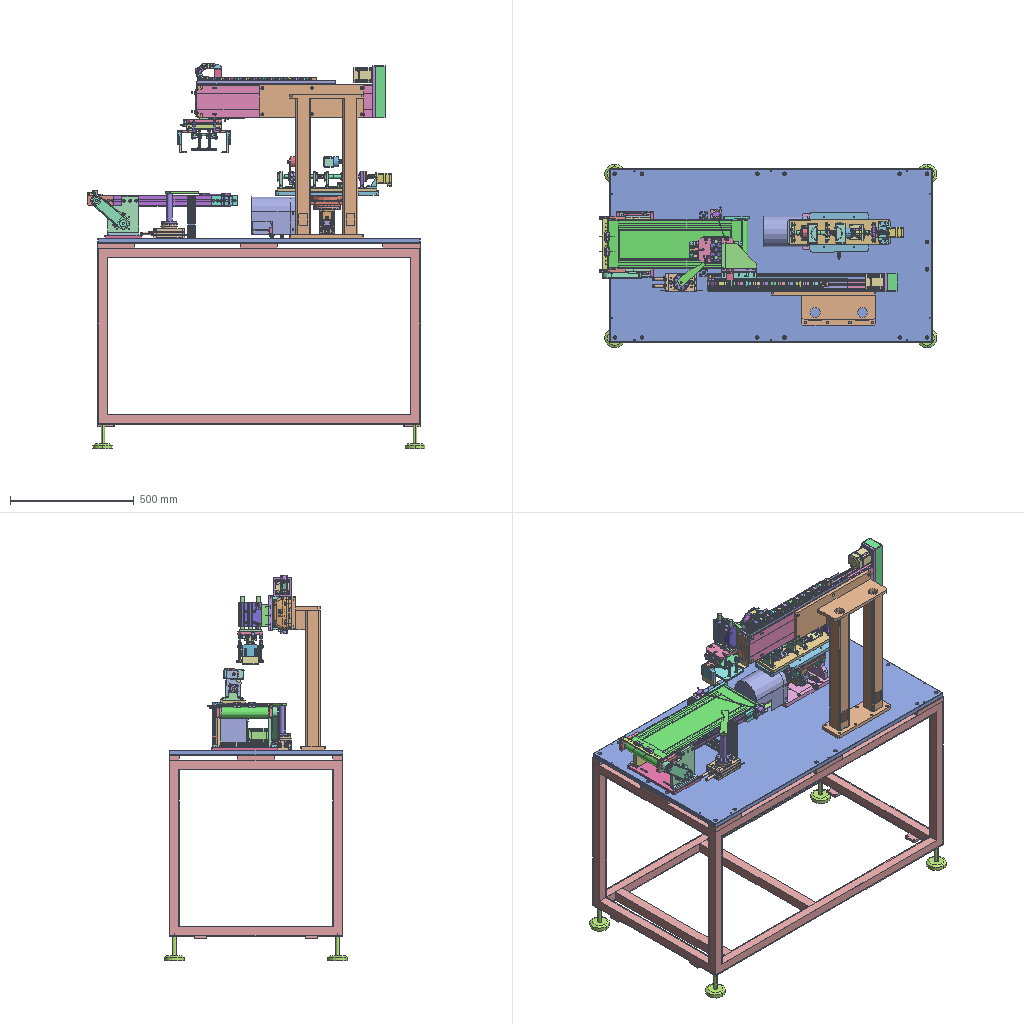Assembly | SolidWorks | 144 different items | 252 placed | box 1362 x 740 x 1556 mm
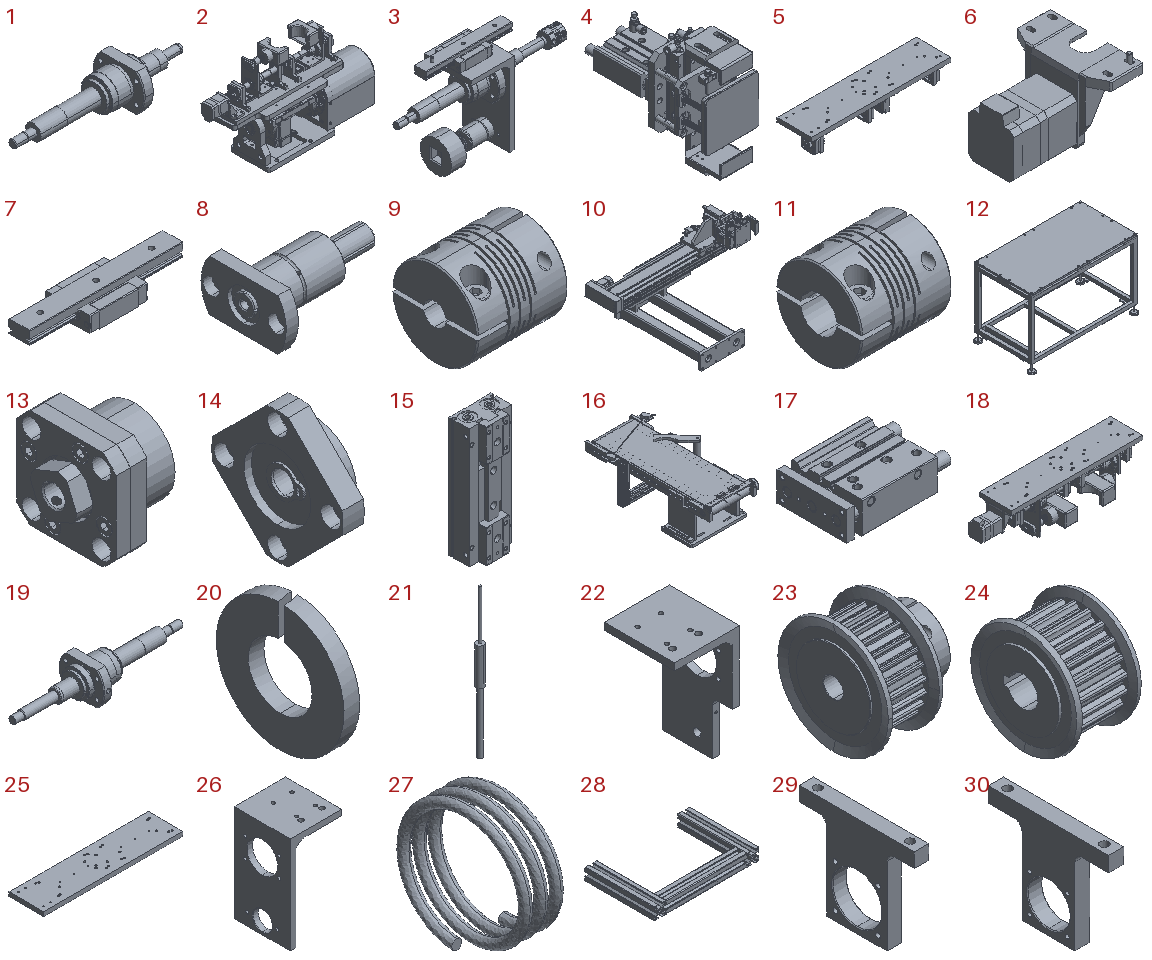Parts list (item | name | quantity | parent item | size | volume | features):
1 | (subassembly) | x1 | in 18 | 171 x 53 x 38 mm | 62164 mm3 | features AEMSimFeature 1
2 | (subassembly) | x1 | - | - | 4755058 mm3 | features CompositeCurve 2, ReferencePattern 2, MirrorCompFeat 1
3 | (subassembly) | x1 | in 18 | 209.2 x 60 x 132 mm | 185380 mm3 | features AEMSimFeature 1, CompositeCurve 1
4 | (subassembly) | x1 | in 10 | 110 x 275 x 215 mm | 1117896 mm3 | features CompositeCurve 3
5 | (subassembly) | x1 | in 18 | 400 x 100 x 81 mm | 622322 mm3 | features AEMSimFeature 1
6 | (subassembly) | x1 | in 18 | 99 x 88 x 69 mm | 136983 mm3 | features AEMSimFeature 1
7 | (subassembly) | x2 | in 3, 18 | 110 x 32 x 16 mm | 26387 mm3 | features AEMSimFeature 1
8 | (subassembly) | x1 | in 3 | 60 x 42 x 25 mm | 18059 mm3 | features AEMSimFeature 1
9 | (subassembly) | x1 | in 3 | 20 x 19 x 19 mm | 4000 mm3 | features AEMSimFeature 1
10 | (subassembly) | x1 | - | - | 8279258 mm3 | -
11 | (subassembly) | x1 | in 18 | 20 x 19 x 19 mm | 3812 mm3 | features AEMSimFeature 1
12 | (subassembly) | x1 | - | 1340 x 740 x 850 mm | 26625287 mm3 | -
13 | (subassembly) | x1 | in 5 | 34.5 x 42 x 42 mm | 32034 mm3 | features AEMSimFeature 1
14 | (subassembly) | x3 | in 5 | 12 x 43 x 43 mm | 8481 mm3 | features AEMSimFeature 1
15 | (subassembly) | x1 | in 4 | 50 x 33 x 142.8 mm | 178016 mm3 | -
16 | (subassembly) | x1 | - | 341.242 x 608 x 194 mm | 3807231 mm3 | features Belt 1
17 | (subassembly) | x1 | in 4 | 142 x 93 x 42 mm | 365239 mm3 | -
18 | (subassembly) | x1 | in 2 | - | 1293275 mm3 | features AEMSimFeature 1, CompositeCurve 1, MateUpdatePoint 1
19 | (subassembly) | x1 | in 3 | 196 x 53 x 38 mm | 63498 mm3 | features AEMSimFeature 1
20 | - | x1 | in 18 | 1.5 x 12.2 x 12.197 mm | 128.674 mm3 | features BaseBody 1
21 | - | x2 | in 16 | 3 x 3 x 60 mm | 185.354 mm3 | features BaseBody 1
22 | - | x1 | in 18 | 55 x 60 x 104 mm | 45466 mm3 | features ICE 5, HoleWzd 3, Fillet 2, Extrusion 1
23 | - | x1 | in 16 | - | - | features BaseBody 1, RefSurface 1
24 | - | x1 | in 16 | 22 x 36 x 36 mm | 13176 mm3 | features BaseBody 1
25 | - | x1 | in 5 | 400 x 100 x 12 mm | 474136 mm3 | features HoleWzd 4, Extrusion 1, ICE 1
26 | - | x1 | in 3 | 55 x 60 x 104 mm | 48156 mm3 | features ICE 3, HoleWzd 2, Chamfer 1, Extrusion 1, Fillet 1
27 | - | x2 | in 3 | 7.3 x 16 x 16 mm | 183.83 mm3 | features BaseBody 1, RefAxis 1
28 | - | x1 | in 16 | 260 x 171 x 30 mm | 182154 mm3 | features WeldMemberFeat 1, WeldmentFeature 1
29 | - | x1 | in 5 | 10 x 80 x 69 mm | 22964 mm3 | features HoleWzd 2, Chamfer 1, Extrusion 1, Fillet 1, ICE 1
30 | - | x3 | in 5 | 10 x 80 x 66 mm | 20856 mm3 | features HoleWzd 2, Chamfer 1, Extrusion 1, Fillet 1, ICE 1
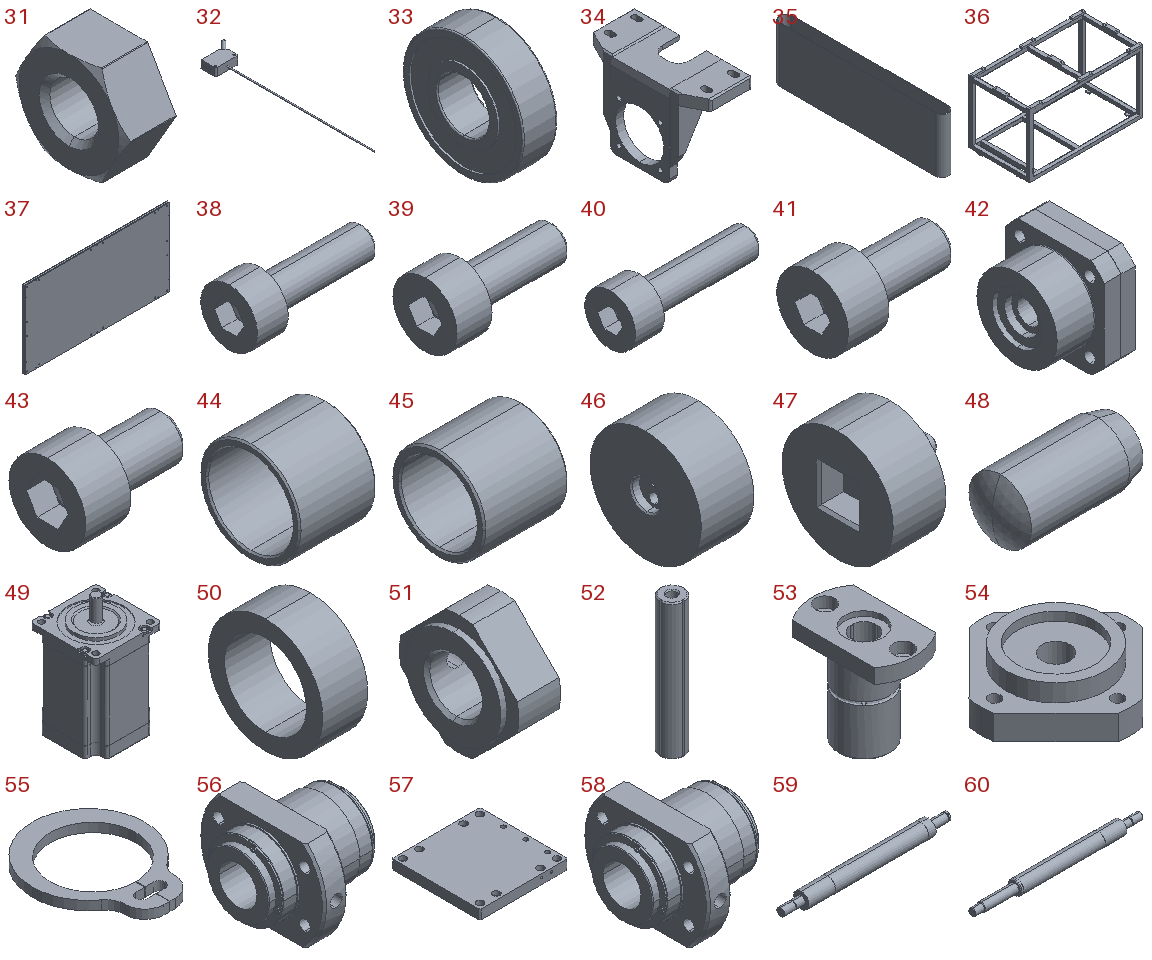31 | - | x1 | in 18 | 5 x 11.5 x 10 mm | 332.083 mm3 | features BaseBody 1
32 | - | x2 | in 16 | 44.556 x 232.556 x 10.8 mm | 6994 mm3 | features BaseBody 1
33 | - | x4 | in 16 | 8 x 28 x 28 mm | 3776 mm3 | features BaseBody 1
34 | - | x1 | in 6 | 40 x 88 x 62 mm | 31074 mm3 | features ICE 9, Chamfer 4, Fillet 3, Extrusion 1, HoleWzd 1
35 | - | x1 | in 16 | 44.5 x 584.5 x 190 mm | 461137 mm3 | features BeltProfileFeature 1, ExtruThin 1
36 | - | x1 | in 12 | 1300 x 700 x 740 mm | 7989139 mm3 | features ICE 11, MirrorPattern 9, HoleWzd 5, LPattern 5, 3DProfileFeature 4, Chamfer 1, Extrusion 1, Shell 1
37 | - | x1 | in 12 | 1300 x 20 x 700 mm | 18144468 mm3 | features MirrorPattern 5, 3DProfileFeature 4, HoleWzd 4, LPattern 4, Chamfer 1, Extrusion 1
38 | - | x8 | in 3, 5, 6, 18 | 13 x 5.5 x 5.5 mm | 132.881 mm3 | features BaseBody 1
39 | - | x1 | in 3 | 11 x 5.5 x 5.5 mm | 118.744 mm3 | features BaseBody 1
40 | - | x4 | in 3, 5, 6, 18 | 19 x 7 x 7 mm | 324.822 mm3 | features BaseBody 1
41 | - | x1 | in 3 | 12 x 7 x 7 mm | 236.857 mm3 | features BaseBody 1
42 | - | x1 | in 13 | 29 x 42 x 42 mm | 30074 mm3 | features BaseBody 1
43 | - | x1 | in 3 | 13 x 8.5 x 8.5 mm | 402.153 mm3 | features BaseBody 1
44 | - | x1 | in 3 | 10 x 13 x 13 mm | 373.975 mm3 | features BaseBody 1
45 | - | x1 | in 18 | 10 x 11 x 11 mm | 311.646 mm3 | features BaseBody 1
46 | - | x1 | in 3 | 19 x 40 x 40 mm | 21751 mm3 | features ICE 3, Chamfer 2, HoleWzd 1, Revolution 1
47 | - | x1 | in 18 | 33 x 40 x 40 mm | 22559 mm3 | features Chamfer 2, ICE 2, Revolution 1
48 | - | x16 | in 3, 5, 18 | 10 x 5 x 5 mm | 185.449 mm3 | features Revolution 1
49 | - | x1 | in 16 | 57.15 x 58.15 x 100.6 mm | 235224 mm3 | features BaseBody 2
50 | - | x1 | in 13 | 5.5 x 14 x 14 mm | 414.69 mm3 | features BaseBody 1
51 | - | x1 | in 13 | 8 x 20 x 20 mm | 1546 mm3 | features BaseBody 1
52 | - | x1 | in 8 | 10.348 x 10.348 x 60 mm | 4741 mm3 | features BaseBody 1
53 | - | x1 | in 8 | 25 x 42 x 40 mm | 13318 mm3 | features BaseBody 1
54 | - | x3 | in 14 | 43 x 43 x 12 mm | 8449 mm3 | features BaseBody 1
55 | - | x3 | in 14 | 10 x 12.2 x 0.8 mm | 32.103 mm3 | features BaseBody 1
56 | - | x1 | in 19 | 45 x 53 x 38 mm | 34023 mm3 | features ICE 5, CirPattern 2, HoleWzd 2, Chamfer 1, Fillet 1, RevCut 1, Revolution 1
57 | - | x1 | in 10 | 140 x 140 x 15 mm | 283192 mm3 | features HoleWzd 3, Chamfer 1, Extrusion 1, LPattern 1, MirrorPattern 1
58 | - | x1 | in 1 | 45 x 53 x 38 mm | 34023 mm3 | features ICE 5, CirPattern 2, HoleWzd 2, Chamfer 1, Fillet 1, RevCut 1, Revolution 1
59 | - | x1 | in 1 | 171 x 16 x 16 mm | 28140 mm3 | features Chamfer 1, RevCut 1, Revolution 1
60 | - | x1 | in 19 | 196 x 16 x 16 mm | 29474 mm3 | features Chamfer 2, RevCut 1, Revolution 1
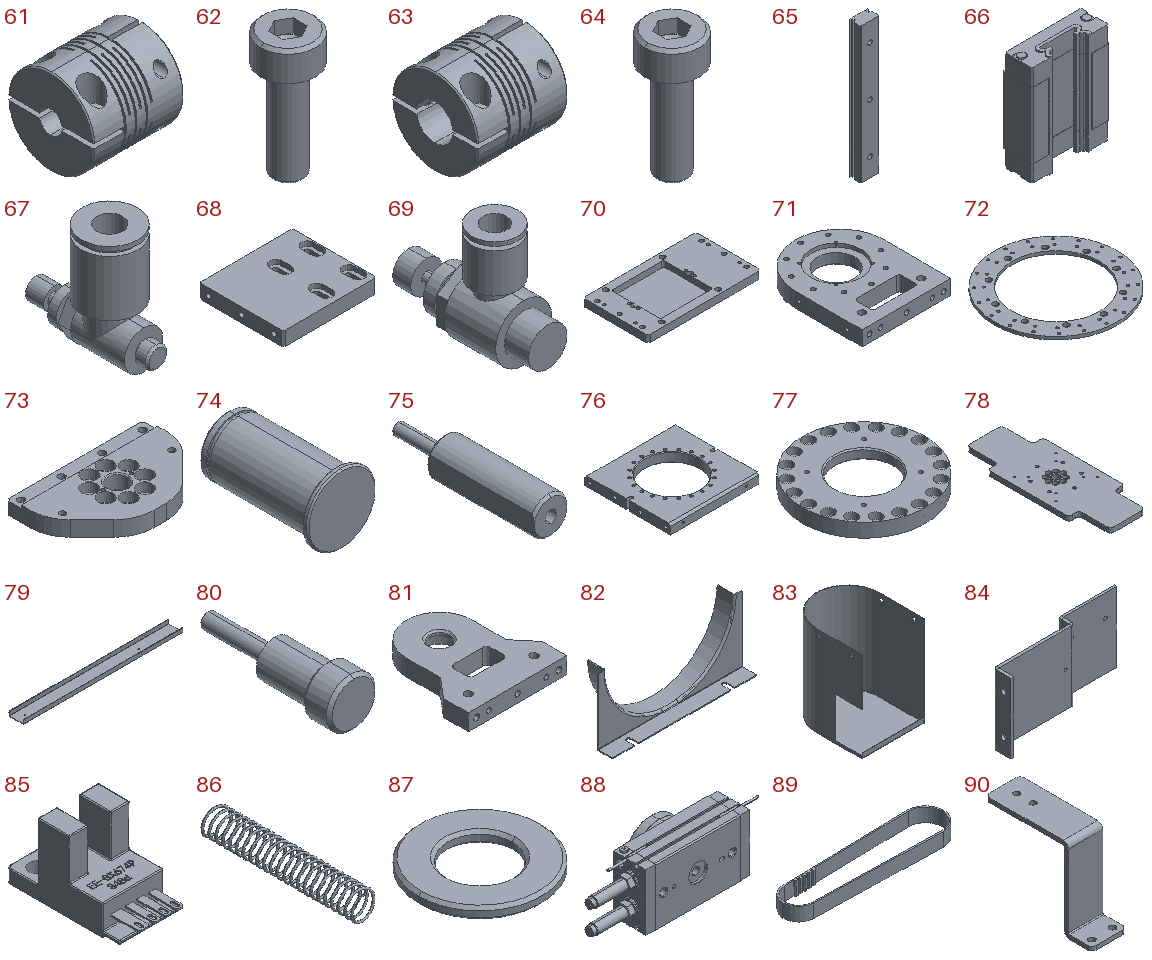61 | - | x1 | in 9 | 20 x 19 x 19 mm | 3713 mm3 | features BaseBody 1
62 | - | x4 | in 9 | 4.5 x 4.5 x 10.36 mm | 71.746 mm3 | features BaseBody 1
63 | - | x1 | in 11 | 20 x 19 x 19 mm | 3525 mm3 | features BaseBody 1
64 | - | x4 | in 11 | 4.5 x 4.5 x 10.36 mm | 71.746 mm3 | features BaseBody 1
65 | - | x2 | in 7 | 15 x 9.5 x 110 mm | 14060 mm3 | features BaseBody 1
66 | - | x2 | in 7 | 32 x 12 x 42.4 mm | 12327 mm3 | features BaseBody 1
67 | - | x2 | in 4 | 13 x 28.3 x 26 mm | 2880 mm3 | features BaseBody 1
68 | - | x1 | in 10 | 100 x 90 x 15 mm | 125181 mm3 | features ICE 2, Chamfer 1, Extrusion 1, HoleWzd 1, LPattern 1
69 | - | x2 | in 4 | 14.2 x 35.2 x 27.5 mm | 4410 mm3 | features BaseBody 1
70 | - | x1 | in 2 | 252 x 145 x 16 mm | 394345 mm3 | features HoleWzd 5, Chamfer 1, Extrusion 1, ICE 1, MirrorPattern 1
71 | - | x1 | in 2 | 120 x 150 x 20 mm | 234004 mm3 | features HoleWzd 6, CirPattern 2, ICE 2, Chamfer 1, Extrusion 1, MirrorPattern 1
72 | - | x2 | in 2 | 123 x 123 x 3 mm | 16511 mm3 | features CirPattern 2, HoleWzd 2, Extrusion 1
73 | - | x2 | in 2 | 135 x 85 x 15 mm | 108283 mm3 | features HoleWzd 5, Chamfer 2, CirPattern 1, Extrusion 1, ICE 1
74 | - | x2 | in 2 | 24 x 40 x 24 mm | 12725 mm3 | features Revolution 1
75 | - | x2 | in 2 | 7 x 33 x 8 mm | 1085 mm3 | features Chamfer 2, Fillet 1, HoleWzd 1, ICE 1, Revolution 1
76 | - | x1 | in 2 | 140 x 135 x 15 mm | 184976 mm3 | features HoleWzd 3, Chamfer 2, MirrorPattern 2, CirPattern 1, Extrusion 1, ICE 1
77 | - | x1 | in 2 | 107 x 107 x 12 mm | 66155 mm3 | features CirPattern 2, HoleWzd 2, Chamfer 1, Extrusion 1, ICE 1
78 | - | x1 | in 2 | 160 x 415 x 14 mm | 752880 mm3 | features HoleWzd 3, CirPattern 2, ICE 2, Chamfer 1, Extrusion 1, Fillet 1, MirrorPattern 1
79 | - | x1 | in 10 | 560 x 52 x 15 mm | 65239 mm3 | features ICE 2, EdgeFlange 1, Fillet 1, FlatPattern 1, HoleWzd 1, LPattern 1, SMBaseFlange 1, SheetMetal 1
80 | - | x1 | in 2 | 8 x 24 x 8 mm | 516.339 mm3 | features Chamfer 2, Fillet 1, Revolution 1
81 | - | x1 | in 2 | 120 x 135 x 20 mm | 181137 mm3 | features HoleWzd 3, ICE 2, Chamfer 1, Extrusion 1
82 | - | x2 | in 2 | 150 x 33 x 69 mm | 8933 mm3 | features ICE 3, Fillet 2, EdgeFlange 1, FlatPattern 1, SMBaseFlange 1, SheetMetal 1
83 | - | x1 | in 2 | 124 x 152 x 178 mm | 79554 mm3 | features EdgeFlange 3, ICE 2, 3DProfileFeature 1, FlatPattern 1, SMBaseFlange 1, SheetMetal 1
84 | - | x1 | in 2 | 151 x 33 x 80 mm | 42488 mm3 | features EdgeFlange 3, HoleWzd 3, FlatPattern 1, SMBaseFlange 1, SheetMetal 1
85 | - | x6 | in 2 | 13.6 x 28 x 16 mm | 2162 mm3 | features ICE 6, Fillet 3, Chamfer 1, Extrusion 1, HoleWzd 1
86 | - | x4 | in 4 | 8 x 45 x 8 mm | 146.9 mm3 | features Helix 1, ICE 1, Sweep 1
87 | - | x1 | in 3 | 21 x 21 x 2 mm | 477.522 mm3 | features BaseBody 1
88 | - | x1 | in 16 | 200 x 57 x 74 mm | 397497 mm3 | features BaseBody 3
89 | - | x1 | in 16 | 177.014 x 40.237 x 15 mm | 9222 mm3 | features BaseBody 1
90 | - | x1 | in 10 | 25 x 77 x 60 mm | 9704 mm3 | features EdgeFlange 2, HoleWzd 2, Fillet 1, FlatPattern 1, SMBaseFlange 1, SheetMetal 1
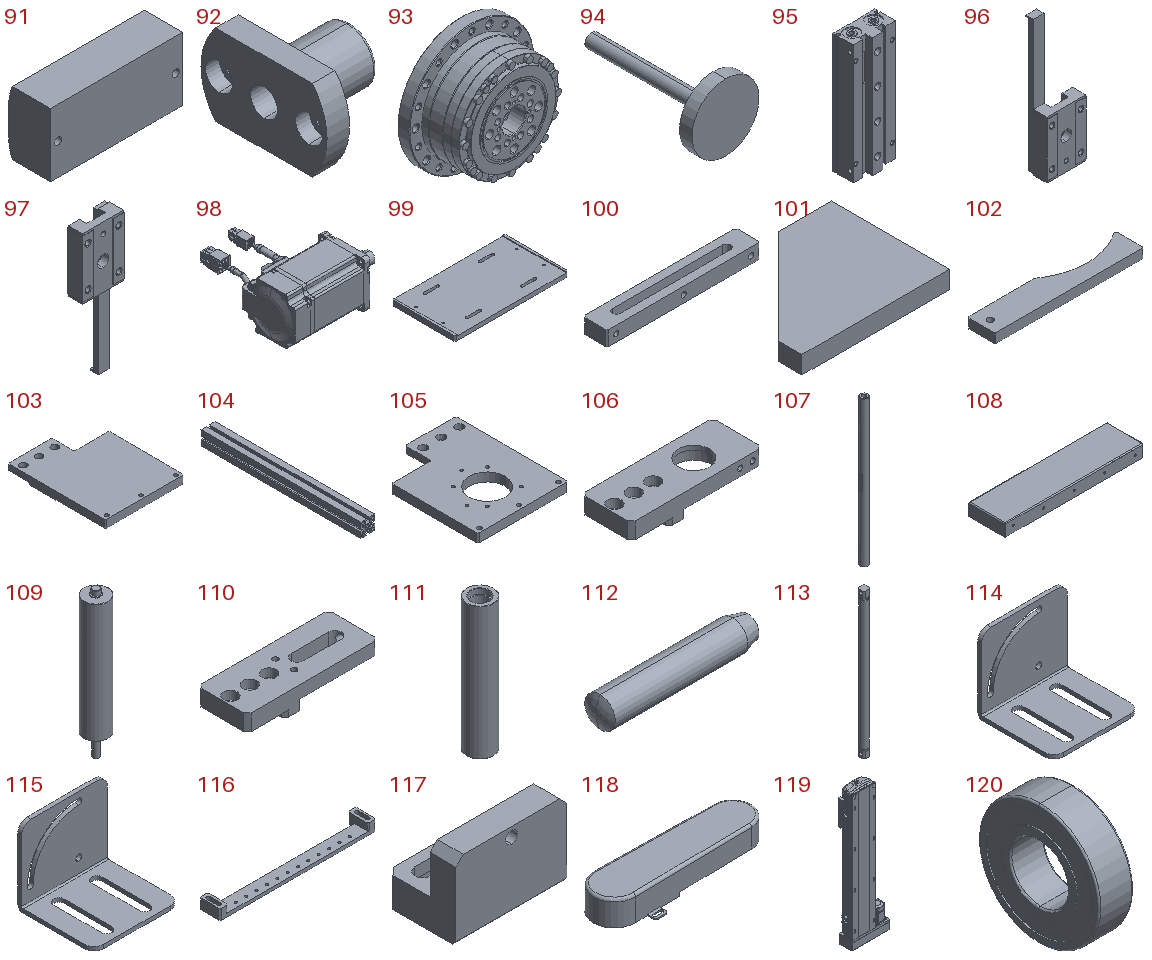91 | - | x1 | in 2 | 77.96 x 24.63 x 37.4 mm | 70032 mm3 | features ICE 3, Extrusion 1
92 | - | x4 | in 4 | 19 x 28 x 18 mm | 3154 mm3 | features RevCut 2, ICE 1, Revolution 1
93 | - | x2 | in 2 | 107 x 52 x 107 mm | 219965 mm3 | features BaseBody 45
94 | - | x4 | in 12 | 80 x 160 x 80 mm | 122920 mm3 | features Revolution 1
95 | - | x1 | in 15 | 50 x 28.3 x 142 mm | 158930 mm3 | features BaseBody 1
96 | - | x1 | in 15 | 27 x 14.6 x 93.2 mm | 9543 mm3 | features BaseBody 1
97 | - | x1 | in 15 | 27 x 14.6 x 93.2 mm | 9543 mm3 | features BaseBody 1
98 | - | x2 | in 2 | 129 x 145.682 x 60 mm | 347582 mm3 | features BaseBody 7
99 | - | x1 | in 16 | 268 x 150 x 12 mm | 394710 mm3 | features ICE 2, Chamfer 1, Extrusion 1, HoleWzd 1
100 | - | x2 | in 16 | 125 x 20 x 12 mm | 22020 mm3 | features Chamfer 2, Extrusion 1, HoleWzd 1, ICE 1
101 | - | x1 | in 10 | 125 x 100 x 15 mm | 139500 mm3 | features Chamfer 1, Extrusion 1
102 | - | x1 | in 16 | 160 x 30 x 10 mm | 39472 mm3 | features Chamfer 2, Extrusion 1, HoleWzd 1, ICE 1
103 | - | x1 | in 16 | 125 x 156 x 12 mm | 198828 mm3 | features HoleWzd 2, ICE 2, Chamfer 1, Extrusion 1, Fillet 1
104 | - | x2 | in 16 | 40 x 455 x 40 mm | 322038 mm3 | features WeldMemberFeat 1, WeldmentFeature 1
105 | - | x1 | in 16 | 125 x 156 x 12 mm | 174396 mm3 | features HoleWzd 4, ICE 3, Chamfer 1, Extrusion 1, Fillet 1
106 | - | x2 | in 16 | 105 x 40 x 18 mm | 43487 mm3 | features ICE 5, HoleWzd 2, Chamfer 1, Extrusion 1, MirrorPattern 1
107 | - | x2 | in 16 | 10 x 10 x 194 mm | 14513 mm3 | features HoleWzd 2, Chamfer 1, Extrusion 1, ICE 1
108 | - | x1 | in 16 | 455 x 120 x 40 mm | 145562 mm3 | features Extrusion 1, Fillet 1, HoleWzd 1, Shell 1
109 | - | x1 | in 16 | 40.5 x 40.5 x 246 mm | 261959 mm3 | features ICE 6, Chamfer 1, Extrusion 1, Fillet 1
110 | - | x2 | in 16 | 105 x 40 x 18 mm | 42827 mm3 | features HoleWzd 3, ICE 3, Chamfer 1, Cut 1, Extrusion 1
111 | - | x1 | in 16 | 40.5 x 40.5 x 200 mm | 157423 mm3 | features ICE 2, Chamfer 1, Extrusion 1, MirrorPattern 1
112 | - | x2 | in 3, 18 | 10 x 2 x 2 mm | 30.238 mm3 | features Revolution 1
113 | - | x1 | in 16 | 12 x 12 x 226 mm | 24710 mm3 | features Extrusion 1, HoleWzd 1, ICE 1, MirrorPattern 1, RevCut 1
114 | - | x1 | in 16 | 45 x 40 x 40 mm | 5977 mm3 | features ICE 2, EdgeFlange 1, Fillet 1, FlatPattern 1, HoleWzd 1, SMBaseFlange 1, SheetMetal 1
115 | - | x1 | in 16 | 45 x 40 x 40 mm | 5977 mm3 | features ICE 2, EdgeFlange 1, Fillet 1, FlatPattern 1, HoleWzd 1, SMBaseFlange 1, SheetMetal 1
116 | - | x1 | in 16 | 226 x 30 x 15 mm | 25281 mm3 | features ICE 4, Chamfer 1, Extrusion 1, Fillet 1, HoleWzd 1, LPattern 1
117 | - | x2 | in 16 | 30 x 19 x 20.5 mm | 5581 mm3 | features ICE 4, Chamfer 2, HoleWzd 2, Extrusion 1
118 | - | x1 | in 16 | 189.5 x 70 x 30 mm | 29758 mm3 | features ICE 3, Extrusion 1, Fillet 1, MirrorPattern 1, Shell 1
119 | - | x1 | in 10 | 224 x 78.028 x 768.474 mm | 3697252 mm3 | features BaseBody 11
120 | - | x1 | in 2 | 12 x 42 x 42 mm | 12378 mm3 | features RefAxis 9, 3DProfileFeature 3, Revolution 1
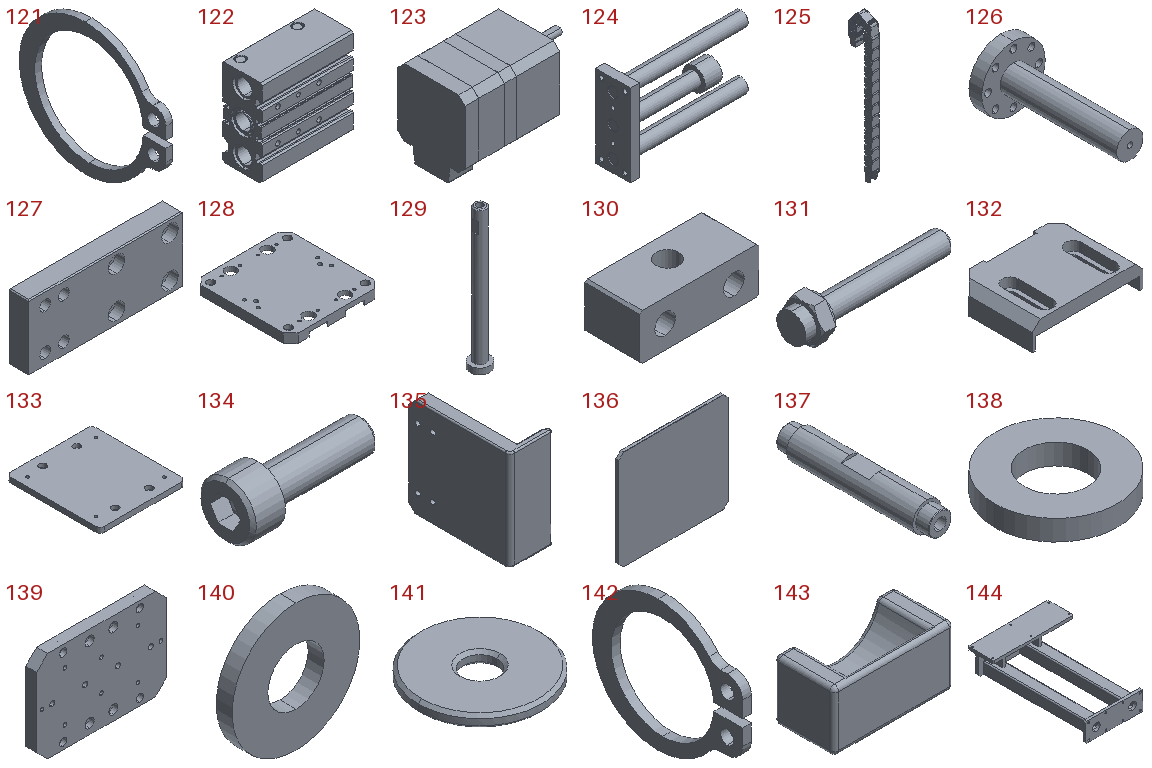121 | - | x1 | in 2 | 1.2 x 25.6 x 23.05 mm | 179.471 mm3 | features RefAxis 6, 3DProfileFeature 2, Extrusion 1, ICE 1
122 | - | x1 | in 17 | 97.5 x 42 x 93 mm | 253511 mm3 | features BaseBody 1
123 | - | x1 | in 6 | 79 x 42 x 51 mm | 105451 mm3 | features ICE 8, Chamfer 1, Extrusion 1, Fillet 1, HoleWzd 1, Revolution 1
124 | - | x1 | in 17 | 142 x 38 x 91 mm | 111727 mm3 | features BaseBody 1
125 | - | x1 | in 10 | 29.1 x 79.262 x 491.255 mm | 146687 mm3 | features BaseBody 18
126 | - | x1 | in 16 | 60 x 126 x 60 mm | 87403 mm3 | features HoleWzd 3, Cut 1, Extrusion 1, ICE 1
127 | - | x2 | in 4 | 75 x 10 x 32 mm | 18437 mm3 | features ICE 3, HoleWzd 2, Chamfer 1, Extrusion 1
128 | - | x1 | in 4 | 100 x 106 x 10 mm | 85872 mm3 | features HoleWzd 4, ICE 3, Chamfer 1, Extrusion 1, MirrorPattern 1
129 | - | x4 | in 4 | 10 x 10 x 71 mm | 2041 mm3 | features ICE 2, Chamfer 1, Extrusion 1, HoleWzd 1
130 | - | x2 | in 4 | 26 x 12 x 10 mm | 2220 mm3 | features HoleWzd 2, Chamfer 1, Extrusion 1
131 | - | x2 | in 4 | 42.15 x 11.547 x 10 mm | 1487 mm3 | features RevCut 4, ICE 2, Chamfer 1, Extrusion 1, Fillet 1, LPattern 1, Revolution 1
132 | - | x2 | in 4 | 70 x 50 x 16 mm | 29528 mm3 | features ICE 4, Chamfer 2, Extrusion 1, HoleWzd 1
133 | - | x1 | in 4 | 100 x 110 x 6 mm | 64666 mm3 | features HoleWzd 2, Extrusion 1, Fillet 1
134 | - | x4 | in 5 | 21 x 8.5 x 8.5 mm | 556.026 mm3 | features BaseBody 1
135 | - | x2 | in 4 | 28 x 67 x 66 mm | 39840 mm3 | features Fillet 3, Chamfer 2, Extrusion 1, HoleWzd 1
136 | - | x1 | in 4 | 110 x 3 x 100 mm | 32835 mm3 | features Chamfer 2, Extrusion 1, HoleWzd 1
137 | - | x4 | in 4 | 10 x 53 x 10 mm | 3526 mm3 | features ICE 3, Chamfer 1, HoleWzd 1, MirrorPattern 1, Revolution 1
138 | - | x8 | in 4 | 12 x 12 x 2 mm | 165.813 mm3 | features Extrusion 1
139 | - | x1 | in 4 | 142 x 12 x 100 mm | 155775 mm3 | features HoleWzd 6, Chamfer 1, Extrusion 1, ICE 1
140 | - | x8 | in 4 | 12 x 1.5 x 12 mm | 136.553 mm3 | features FlatPattern 1, SMBaseFlange 1, SheetMetal 1
141 | - | x1 | in 3 | 20 x 20 x 2 mm | 560.774 mm3 | features BaseBody 1
142 | - | x2 | in 16 | 1 x 16.8 x 14.65 mm | 77.172 mm3 | features BaseBody 1
143 | - | x2 | in 18 | 80 x 40 x 40 mm | 93219 mm3 | features Extrusion 1, Fillet 1, ICE 1
144 | - | x1 | in 10 | 420 x 620 x 135 mm | 2694672 mm3 | features ICE 7, Chamfer 3, LPattern 2, Extrusion 1, HoleWzd 1
Mates (type | each side: item.copy, entity, surface, feature), first 302 of 527 lines:
In the top assembly
Coincident | 37.1 face plane Boss-Extrude 1 | 70.1 face plane Boss-Extrude 1
Coincident | 37.1 face plane Boss-Extrude 1 | 144.1 face plane Boss-Extrude 1
DistanceDim | 144.1 face plane Boss-Extrude 1 | 37.1 face plane Boss-Extrude 1 | 2 times
DistanceDim | 70.1 face plane Boss-Extrude 1 | 36.1 face plane Boss-Extrude 1
DistanceDim | 81.1 face plane Boss-Extrude 1 | 37.1 face plane Boss-Extrude 1
Coincident | 37.1 face plane Boss-Extrude 1 | 99.1 face plane Boss-Extrude 1
DistanceDim | 99.1 face plane Boss-Extrude 1 | 36.1 face plane Boss-Extrude 1
DistanceDim | 103.1 face plane Boss-Extrude 1 | 37.1 face plane Boss-Extrude 1
In subassembly 12
DistanceDim | 36.2 face plane Boss-Extrude 1 | 37.2 face plane Boss-Extrude 1
Coincident | 36.2 face plane Boss-Extrude 1 | 37.2 face plane Boss-Extrude 1 | 2 times
DistanceDim | 94.1 face plane Revolve 1 | 36.2 face plane Boss-Extrude 2
Concentric | 36.2 face cylinder Mirror 3 | 94.1 face cylinder Revolve 1
Coincident | 94.1 face plane Revolve 1 | 94.2 face plane Revolve 1
Coincident | 94.1 face plane Revolve 1 | 94.3 face plane Revolve 1
Coincident | 94.2 face plane Revolve 1 | 94.4 face plane Revolve 1
Concentric | 36.2 face cylinder Mirror 4 | 94.4 face cylinder Revolve 1
Concentric | 36.2 face cylinder Mirror 4 | 94.2 face cylinder Revolve 1
Concentric | 36.2 face cylinder Boss-Extrude 8 | 94.3 face cylinder Revolve 1
In subassembly 16
Coincident | 100.1 face plane Boss-Extrude 1 | 103.2 face plane Boss-Extrude 1 | 3 times
Coincident | 99.2 face plane Cut-Extrude 1 | 100.1 face plane Boss-Extrude 1 | 2 times
Width | 99.2 face plane Boss-Extrude 1 | 99.2 face plane Boss-Extrude 1 | 100.1 face plane Boss-Extrude 1 | 100.1 face plane Boss-Extrude 1
Coincident | 105.1 face plane Boss-Extrude 1 | 100.2 face plane Boss-Extrude 1 | 3 times
Coincident | 99.2 face plane Cut-Extrude 1 | 105.1 face plane Boss-Extrude 1
Width | 99.2 face plane Boss-Extrude 1 | 99.2 face plane Boss-Extrude 1 | 100.2 face plane Boss-Extrude 1 | 100.2 face plane Boss-Extrude 1
Coincident | 99.2 face plane Cut-Extrude 1 | 100.2 face plane Boss-Extrude 1
Coincident | 106.1 face plane Cut-Extrude 1 | 104.1 face plane Dongye Aluminium Profile EF4040(1) | 2 times
Width | 104.1 face plane Dongye Aluminium Profile EF4040(1) | 104.1 face plane Dongye Aluminium Profile EF4040(1) | 106.1 face plane Boss-Extrude 1 | 106.1 face plane Boss-Extrude 1
Coincident | 103.2 face plane Cut-Extrude 2 | 104.1 face plane Dongye Aluminium Profile EF4040(1) | 2 times
Coincident | 104.1 face plane Dongye Aluminium Profile EF4040(1) | 104.2 face plane Dongye Aluminium Profile EF4040(1) | 2 times
Coincident | 105.1 face plane Cut-Extrude 2 | 104.2 face plane Dongye Aluminium Profile EF4040(1)
Coincident | 106.2 face plane Cut-Extrude 1 | 104.2 face plane Dongye Aluminium Profile EF4040(1) | 2 times
Width | 104.2 face plane Dongye Aluminium Profile EF4040(1) | 104.2 face plane Dongye Aluminium Profile EF4040(1) | 106.2 face plane Boss-Extrude 1 | 106.2 face plane Boss-Extrude 1
Concentric | 106.1 face cylinder Cut-Extrude 3 | 107.1 face cylinder Boss-Extrude 1
Width | 106.2 face plane Cut-Extrude 3 | 106.1 face plane Cut-Extrude 3 | 107.1 face plane Boss-Extrude 1 | 107.1 face plane Boss-Extrude 1
Coincident | 104.2 face plane Dongye Aluminium Profile EF4040(1) | 108.1 face plane Boss-Extrude 1
Width | 104.2 face plane Dongye Aluminium Profile EF4040(1) | 104.1 face plane Dongye Aluminium Profile EF4040(1) | 108.1 face plane Boss-Extrude 1 | 108.1 face plane Boss-Extrude 1
Coincident | 104.1 face plane Dongye Aluminium Profile EF4040(1) | 108.1 face plane Boss-Extrude 1
Concentric | 106.1 face cylinder Cut-Extrude 4 | 33.1 face cylinder Import 1
Coincident | 106.1 face plane Cut-Extrude 4 | 33.1 face plane Import 1
Concentric | 106.2 face cylinder Cut-Extrude 4 | 33.2 face cylinder Import 1
Coincident | 106.2 face plane Cut-Extrude 4 | 33.2 face plane Import 1
DistanceDim | 106.2 face plane Boss-Extrude 1 | 105.1 face plane Cut-Extrude 1
Concentric | 33.1 face cylinder Import 1 | 109.1 face cylinder Boss-Extrude 4
Coincident | 33.1 face plane Import 1 | 109.1 face plane Boss-Extrude 3
Coincident | 104.2 face plane Dongye Aluminium Profile EF4040(1) | 110.1 face plane Cut-Extrude 1 | 2 times
Width | 104.2 face plane Dongye Aluminium Profile EF4040(1) | 104.2 face plane Dongye Aluminium Profile EF4040(1) | 110.1 face plane Boss-Extrude 1 | 110.1 face plane Boss-Extrude 1
Coincident | 104.1 face plane Dongye Aluminium Profile EF4040(1) | 110.2 face plane Cut-Extrude 1 | 2 times
Width | 104.1 face plane Dongye Aluminium Profile EF4040(1) | 104.1 face plane Dongye Aluminium Profile EF4040(1) | 110.2 face plane Boss-Extrude 1 | 110.2 face plane Boss-Extrude 1
Width | 110.2 face plane Cut-Extrude 3 | 110.1 face plane Cut-Extrude 3 | 107.2 face plane Boss-Extrude 1 | 107.2 face plane Boss-Extrude 1
Concentric | 110.1 face cylinder Cut-Extrude 3 | 107.2 face cylinder Boss-Extrude 1
Concentric | 111.1 face cylinder Mirror 1 | 33.3 face cylinder Import 1
Coincident | 111.1 face plane Mirror 1 | 33.3 face plane Import 1
Concentric | 111.1 face cylinder Cut-Extrude 1 | 33.4 face cylinder Import 1
Coincident | 111.1 face plane Cut-Extrude 1 | 33.4 face plane Import 1
Width | 33.4 face plane Import 1 | 33.3 face plane Import 1 | 113.1 face plane Cut-Revolve 1 | 113.1 face plane Cut-Revolve 1
Concentric | 33.3 face cylinder Import 1 | 113.1 face cylinder Boss-Extrude 1
Coincident | 110.1 face plane Cut-Extrude 4 | 113.1 face plane Cut-Extrude 1
Width | 110.2 face plane Boss-Extrude 1 | 110.1 face plane Boss-Extrude 1 | 113.1 face plane Boss-Extrude 1 | 113.1 face plane Boss-Extrude 1
DistanceDim | 113.1 face plane Cut-Extrude 1 | 110.1 face plane Boss-Extrude 1
Concentric | 113.1 face cylinder Cut-Revolve 1 | 142.1 face cylinder Import 1
Coincident | 33.3 face plane Import 1 | 142.1 face plane Import 1
Parallel | 113.1 plane | 142.1 face plane Import 1
Concentric | 113.1 face cylinder Cut-Revolve 1 | 142.2 face cylinder Import 1
Coincident | 33.4 face plane Import 1 | 142.2 face plane Import 1
Parallel | 113.1 plane | 142.2 face plane Import 1
Concentric | 105.1 face cylinder Cut-Extrude 3 | 49.1 face cylinder Import 1
Coincident | 105.1 face plane Boss-Extrude 1 | 49.1 face plane Import 1
Parallel | 99.2 face plane Cut-Extrude 1 | 49.1 face plane Import 1
Concentric | 49.1 face cylinder Import 2 | 23.1 face cylinder Import 1
Concentric | 109.1 face cylinder Boss-Extrude 6 | 24.1 face cylinder Import 1
Width | 23.1 face plane Import 1 | 23.1 face plane Import 1 | 24.1 face plane Import 1 | 24.1 face plane Import 1
Coincident | 109.1 face plane Boss-Extrude 6 | 24.1 face plane Import 1
Coincident | 109.1 face plane Cut-Extrude 1 | 24.1 face plane Import 1
Concentric | 23.1 face cylinder Import 1 | 89.1 face cylinder Import 1
Width | 23.1 face plane Import 1 | 23.1 face plane Import 1 | 89.1 face plane Import 1 | 89.1 face plane Import 1
Coincident | 23.1 plane | 89.1 plane
PlanarAngleDim | 89.1 face plane Import 1 | 106.2 face plane Boss-Extrude 1
BeltDim | 109.1 face cylinder Boss-Extrude 1 | 111.1 face cylinder Boss-Extrude 1
Coincident | 104.1 face plane Dongye Aluminium Profile EF4040(1) | 114.1 face plane Base-Flange 1
Coincident | 114.1 face plane Edge-Flange 1 | 32.1 face plane Import 1
Concentric | 114.1 face cylinder M3 Clearance Hole 1 | 32.1 face cylinder Import 1
Parallel | 35.1 face plane Extrude-Thin-Walled 1 | 114.1 face plane Edge-Flange 1
Concentric | 32.1 face cylinder Import 1 | 32.2 face cylinder Import 1
Coincident | 32.2 face plane Import 1 | 115.1 face plane Edge-Flange 1
Coincident | 110.1 face plane Boss-Extrude 1 | 115.1 face plane Base-Flange 1
DistanceDim | 115.1 face plane Base-Flange 1 | 110.1 face plane Boss-Extrude 1
Coincident | 110.1 face plane Boss-Extrude 1 | 115.1 face plane Edge-Flange 1
Concentric | 32.2 face cylinder Import 1 | 115.1 face cylinder M3 Clearance Hole 1
DistanceDim | 114.1 face plane Base-Flange 1 | 110.2 face plane Boss-Extrude 1
Coincident | 106.1 face plane Boss-Extrude 1 | 116.1 face plane Boss-Extrude 1
Width | 106.2 face plane Boss-Extrude 1 | 106.1 face plane Boss-Extrude 1 | 116.1 face plane Boss-Extrude 1 | 116.1 face plane Boss-Extrude 1
Coincident | 116.1 face plane Boss-Extrude 1 | 117.1 face plane Cut-Extrude 1 | 2 times
Coincident | 116.1 face plane Boss-Extrude 1 | 117.2 face plane Cut-Extrude 1 | 2 times
DistanceDim | 117.1 face plane Boss-Extrude 1 | 117.2 face plane Boss-Extrude 1
Width | 116.1 face plane Boss-Extrude 1 | 116.1 face plane Boss-Extrude 1 | 117.1 face plane Boss-Extrude 1 | 117.2 face plane Boss-Extrude 1
Concentric | 117.1 face cylinder M3 Clearance Hole 1 | 21.1 face cylinder Import 1
Coincident | 117.1 face plane Boss-Extrude 1 | 21.1 face plane Import 1
Concentric | 117.2 face cylinder M3 Clearance Hole 1 | 21.2 face cylinder Import 1
Coincident | 117.2 face plane Boss-Extrude 1 | 21.2 face plane Import 1
Coincident | 106.2 face plane Boss-Extrude 1 | 116.1 face plane Boss-Extrude 1
Concentric | 23.1 face cylinder Import 1 | 118.1 face cylinder Shell 1
Parallel | 89.1 face plane Import 1 | 118.1 face plane Shell 1
Coincident | 105.1 face plane Boss-Extrude 1 | 118.1 face plane Boss-Extrude 1
Coincident | 104.2 face plane Dongye Aluminium Profile EF4040(1) | 28.1 face plane Aluminium Profile Library 30X 30G X R1.5(1) | 2 times
DistanceDim | 99.2 face plane Boss-Extrude 1 | 28.1 face plane Aluminium Profile Library 30X 30G X R1.5(1)
Coincident | 99.2 face plane Boss-Extrude 1 | 88.1 face plane HRQ30-A_part-1-solid1
DistanceDim | 88.1 face plane HRQ30-A_part-1-solid1 | 99.2 face plane Boss-Extrude 1
Concentric | 88.1 face cylinder HRQ30-A_part-1-solid1 | 126.1 face cylinder Boss-Extrude 1
Coincident | 88.1 face plane HRQ30-A_part-1-solid1 | 126.1 face plane Boss-Extrude 1
Concentric | 88.1 face cylinder HRQ30-A_part-1-solid1 | 126.1 face cylinder M6 Clearance Hole 1
Coincident | 126.1 face plane Boss-Extrude 1 | 102.1 face plane Boss-Extrude 1
Concentric | 126.1 face cylinder M6 Tapped Hole 1 | 102.1 face cylinder M6 Clearance Hole 1
In subassembly 2
Concentric | 70.2 face cylinder Hole Size (% per) Hex Socket Cap Screw Type 2 | 71.1 face cylinder M8 Tapped Hole 1 | 2 times
Coincident | 70.2 face plane Boss-Extrude 1 | 71.1 face plane Boss-Extrude 1
Concentric | 71.1 face cylinder CirPattern 1 | 98.1 face cylinder _MSMF04NoWith key_b.stp-1-solid1 | 2 times
Coincident | 71.1 face plane Boss-Extrude 1 | 98.1 face plane _MSMF04NoWith key_b.stp-1-solid1
Concentric | 71.1 face cylinder Hole Size (% per) Hex Socket Cap Screw Type 2 | 93.1 face cylinder LSS-25-U-I(1).stp-1/ADMI7ED1CHEZ_ASM.stp-1/MANIFOLD_SOLID_BREP_427.stp-1-solid1
Concentric | 71.1 face cylinder CirPattern 2 | 93.1 face cylinder LSS-25-U-I(1).stp-1/ADMI7ED1CHEZ_ASM.stp-1/MANIFOLD_SOLID_BREP_427.stp-1-solid1
Coincident | 71.1 face plane Boss-Extrude 1 | 93.1 face plane LSS-25-U-I(1).stp-1/ADMI7ED1CHEZ_ASM.stp-1/MANIFOLD_SOLID_BREP_427.stp-1-solid1
Concentric | 93.1 face cylinder LSS-25-U-I(1).stp-1/ADMI7ED1CHEZ_ASM.stp-1/MANIFOLD_SOLID_BREP_427.stp-1-solid1 | 72.1 face cylinder CirPattern 1 | 2 times
Coincident | 93.1 face plane LSS-25-U-I(1).stp-1/ADMI7ED1CHEZ_ASM.stp-1/MANIFOLD_SOLID_BREP_427.stp-1-solid1 | 72.1 face plane Boss-Extrude 1
Coincident | 72.1 face plane Boss-Extrude 1 | 85.1 face plane Boss-Extrude 1
Coincident | 72.1 face plane Boss-Extrude 1 | 85.2 face plane Boss-Extrude 1
Coincident | 72.1 face plane Boss-Extrude 1 | 85.3 face plane Boss-Extrude 1
Coincident | 93.1 face plane LSS-25-U-I(1).stp-1/ADMI7ED1CHEZ_ASM.stp-1/MANIFOLD_SOLID_BREP_412.stp-1-solid1 | 73.1 face plane Boss-Extrude 1
Concentric | 73.1 face cylinder Boss-Extrude 1 | 74.1 face cylinder Revolve 1
Coincident | 73.1 face plane Boss-Extrude 1 | 74.1 face plane Revolve 1
Coincident | 73.1 edge | 75.1 face plane Revolve 1
Concentric | 73.1 face cylinder Ø8.0 (8) DiameterHole 1 | 75.1 face cylinder Revolve 1
Coincident | 73.1 edge | 75.2 face plane Revolve 1
Concentric | 73.1 face cylinder Ø8.0 (8) DiameterHole 1 | 75.2 face cylinder Revolve 1
Concentric | 93.1 face cylinder LSS-25-U-I(1).stp-1/ADMI7ED1CHEZ_ASM.stp-1/MANIFOLD_SOLID_BREP_412.stp-1-solid1 | 73.1 face cylinder Boss-Extrude 1
Concentric | 72.1 face cylinder CirPattern 2 | 85.1 face cylinder Ø3.5 (3.5) DiameterHole 1 | 2 times
Concentric | 72.1 face cylinder CirPattern 2 | 85.2 face cylinder Ø3.5 (3.5) DiameterHole 1 | 2 times
Concentric | 72.1 face cylinder CirPattern 2 | 85.3 face cylinder Ø3.5 (3.5) DiameterHole 1 | 2 times
Coincident | 73.1 face plane Cut-Extrude 1 | 76.1 face plane Boss-Extrude 1
Concentric | 73.1 face cylinder Hole Size (% per) Hex Socket Cap Screw Type 3 | 76.1 face cylinder M6 Tapped Hole 1 | 2 times
Concentric | 76.1 face cylinder CirPattern 1 | 93.2 face cylinder LSS-25-U-I(1).stp-1/ADMI7ED1CHEZ_ASM.stp-1/MANIFOLD_SOLID_BREP_427.stp-1-solid1
Concentric | 76.1 face cylinder M5 Tapped Hole 1 | 93.2 face cylinder LSS-25-U-I(1).stp-1/ADMI7ED1CHEZ_ASM.stp-1/MANIFOLD_SOLID_BREP_427.stp-1-solid1
Coincident | 76.1 face plane Boss-Extrude 1 | 93.2 face plane LSS-25-U-I(1).stp-1/ADMI7ED1CHEZ_ASM.stp-1/MANIFOLD_SOLID_BREP_427.stp-1-solid1
Concentric | 77.1 face cylinder Hole Size (% per) Hex Socket Cap Screw Type 1 | 93.2 face cylinder LSS-25-U-I(1).stp-1/ADMI7ED1CHEZ_ASM.stp-1/MANIFOLD_SOLID_BREP_427.stp-1-solid1
Concentric | 77.1 face cylinder CirPattern 1 | 93.2 face cylinder LSS-25-U-I(1).stp-1/ADMI7ED1CHEZ_ASM.stp-1/MANIFOLD_SOLID_BREP_427.stp-1-solid1
Coincident | 93.2 face plane LSS-25-U-I(1).stp-1/ADMI7ED1CHEZ_ASM.stp-1/MANIFOLD_SOLID_BREP_427.stp-1-solid1 | 77.1 face plane Boss-Extrude 1
Concentric | 77.1 face cylinder CirPattern 2 | 98.2 face cylinder _MSMF04NoWith key_b.stp-1-solid1 | 2 times
Coincident | 77.1 face plane Boss-Extrude 1 | 98.2 face plane _MSMF04NoWith key_b.stp-1-solid1
Coincident | 93.2 face plane LSS-25-U-I(1).stp-1/ADMI7ED1CHEZ_ASM.stp-1/MANIFOLD_SOLID_BREP_412.stp-1-solid1 | 78.1 face plane Boss-Extrude 1
Coincident | 72.2 face plane Boss-Extrude 1 | 85.4 face plane Boss-Extrude 1
Coincident | 72.2 face plane Boss-Extrude 1 | 85.5 face plane Boss-Extrude 1
Coincident | 72.2 face plane Boss-Extrude 1 | 85.6 face plane Boss-Extrude 1
Concentric | 72.2 face cylinder CirPattern 2 | 85.6 face cylinder Ø3.5 (3.5) DiameterHole 1 | 2 times
Concentric | 72.2 face cylinder CirPattern 2 | 85.4 face cylinder Ø3.5 (3.5) DiameterHole 1 | 2 times
Concentric | 72.2 face cylinder CirPattern 2 | 85.5 face cylinder Ø3.5 (3.5) DiameterHole 1 | 2 times
Coincident | 76.1 face plane Boss-Extrude 1 | 72.2 face plane Boss-Extrude 1
Concentric | 78.1 face cylinder CirPattern 2 | 80.1 face cylinder Revolve 1
Concentric | 81.2 face cylinder Boss-Extrude 1 | 120.1 face cylinder Revolve 1
Coincident | 81.2 face plane Cut-Extrude 1 | 120.1 face plane Revolve 1
Concentric | 70.2 face cylinder Mirror 1 | 81.2 face cylinder M8 Tapped Hole 1 | 2 times
Coincident | 70.2 face plane Boss-Extrude 1 | 81.2 face plane Boss-Extrude 1
Concentric | 71.1 face cylinder Boss-Extrude 1 | 83.1 face cylinder Edge-Flange 2
Parallel | 71.1 face plane Boss-Extrude 1 | 83.1 face plane Edge-Flange 1
Coincident | 71.1 face plane Boss-Extrude 1 | 83.1 face plane Edge-Flange 1
Concentric | 70.2 face cylinder M6 Tapped Hole 2 | 84.1 face cylinder Ø6.5 (6.5) DiameterHole 2 | 2 times
Coincident | 70.2 face plane Boss-Extrude 1 | 84.1 face plane Edge-Flange 3
Concentric | 84.1 face cylinder M4 Tapped Hole 1 | 91.1 face cylinder Cut-Extrude 2 | 2 times
Coincident | 84.1 face plane Base-Flange 1 | 91.1 face plane Boss-Extrude 1
LimitPlanarAngleDim | 78.1 face plane Boss-Extrude 1 | 70.2 face plane Boss-Extrude 1
Concentric | 76.1 face cylinder Boss-Extrude 1 | 72.2 face cylinder Boss-Extrude 1
Coincident | 78.1 face plane CirPattern 2 | 80.1 face plane Revolve 1
Concentric | 76.1 face cone Chamfer 1 | 82.1 face cylinder Boss-Extrude 1
DistanceDim | 76.1 face plane Boss-Extrude 1 | 82.1 face plane Base-Flange 1
Parallel | 76.1 face plane Boss-Extrude 1 | 82.1 face plane Edge-Flange 1
Concentric | 76.1 face cone Chamfer 1 | 82.2 face cylinder Boss-Extrude 1
Coincident | 82.1 face plane Base-Flange 1 | 82.2 face plane Base-Flange 1
Parallel | 76.1 face plane Boss-Extrude 1 | 82.2 face plane Edge-Flange 1
Concentric | 93.2 face cylinder LSS-25-U-I(1).stp-1/ADMI7ED1CHEZ_ASM.stp-1/MANIFOLD_SOLID_BREP_412.stp-1-solid1 | 78.1 face cylinder Boss-Extrude 1
Coincident | 74.2 face plane Revolve 1 | 121.1 face plane Boss-Extrude 1
Concentric | 74.2 face cylinder Revolve 1 | 121.1 face cylinder Boss-Extrude 1
Coincident | 78.1 face plane Boss-Extrude 1 | 25.1 face plane Boss-Extrude1
Width | 78.1 face plane Boss-Extrude 1 | 78.1 face plane Boss-Extrude 1 | 25.1 face plane Boss-Extrude1 | 25.1 face plane Boss-Extrude1
Width | 25.1 face plane Boss-Extrude1 | 25.1 face plane Boss-Extrude1 | 78.1 face plane Boss-Extrude 1 | 78.1 face plane Boss-Extrude 1
In subassembly 18
Coincident | 25.2 face plane Boss-Extrude1 | 34.1 face plane Boss-Extrude1 | 2 times
Coincident | 25.2 face plane Boss-Extrude1 | 65.1 face plane Imported1
Concentric | 25.2 face cylinder M3 Tapped Hole1 | 65.1 face cylinder Imported1 | 2 times
Concentric | 123.1 face cylinder Revolve1 | 61.1 face cylinder Imported1
Concentric | 25.2 face cylinder M4 Tapped Hole1 | 40.1 face cylinder Imported1
Concentric | 66.1 face cylinder Imported1 | 22.1 face cylinder M4 Tapped Hole1 | 2 times
Coincident | 66.1 face plane Imported1 | 22.1 face plane Boss-Extrude1
Concentric | 65.2 face cylinder Imported1 | 38.1 face cylinder Imported1
Coincident | 65.2 face plane Imported1 | 38.1 edge
Concentric | 59.1 face cylinder Revolve1 | 63.1 face cylinder Imported1
DistanceDim | 59.1 face plane Revolve1 | 63.1 face plane Imported1
Concentric | 22.1 face cylinder Cut-Extrude2 | 48.1 face cylinder Revolve1
Coincident | 22.1 face plane Boss-Extrude1 | 48.1 face plane Revolve1
Concentric | 22.1 face cylinder Cut-Extrude2 | 48.2 face cylinder Revolve1
Coincident | 22.1 face plane Boss-Extrude1 | 48.2 face plane Revolve1
Concentric | 59.1 face cylinder Revolve1 | 45.1 face cylinder Imported1
Coincident | 59.1 face plane Revolve1 | 45.1 face plane Imported1
Concentric | 22.1 face cylinder Cut-Extrude3 | 58.1 face cylinder Revolve1
Coincident | 58.1 face plane Revolve1 | 22.1 face plane Cut-Extrude1
Concentric | 58.1 face cylinder Ø4.5 (4.5) Diameter Hole1 | 40.2 face cylinder Imported1
Coincident | 58.1 face plane Revolve1 | 40.2 face plane Imported1
Concentric | 58.1 face cylinder Ø4.5 (4.5) Diameter Hole1 | 22.1 face cylinder M4 Tapped Hole2
Concentric | 22.1 face cylinder Ø6.5 (6.5) Diameter Hole1 | 47.1 face cylinder Revolve1
Parallel | 22.1 face plane Cut-Extrude4 | 47.1 plane
Coincident | 22.1 face plane Cut-Extrude1 | 47.1 face plane Revolve1
Concentric | 47.1 face cylinder Revolve1 | 20.1 face cylinder Imported1
Concentric | 47.1 face cylinder Revolve1 | 31.1 face cylinder Imported1
Concentric | 22.1 face cylinder Cut-Extrude5 | 112.1 face cylinder Revolve1
DistanceDim | 112.1 face plane Revolve1 | 22.1 face plane Cut-Extrude4
Coincident | 22.1 face plane Boss-Extrude1 | 20.1 face plane Imported1
Concentric | 22.1 face cylinder M4 Tapped Hole1 | 38.2 face cylinder Imported1
Coincident | 22.1 face plane Boss-Extrude1 | 38.2 face plane Imported1
Coincident | 20.1 face plane Imported1 | 31.1 face plane Imported1
Concentric | 25.2 face cylinder M3 Tapped Hole1 | 65.2 face cylinder Imported1 | 2 times
Coincident | 25.2 face plane Boss-Extrude1 | 65.2 face plane Imported1
DistanceDim | 59.1 face plane Revolve1 | 54.1 face plane Imported1
Coincident | 46.1 face plane Revolve1 | 143.1 face plane Boss-Extrude 1
Width | 143.1 face plane Boss-Extrude 1 | 143.1 face plane Boss-Extrude 1 | 26.1 face plane Boss-Extrude1 | 26.1 face plane Boss-Extrude1
Width | 143.1 face plane Boss-Extrude 1 | 143.1 face plane Boss-Extrude 1 | 46.1 face cylinder Revolve1
Coincident | 47.1 face plane Revolve1 | 143.2 face plane Boss-Extrude 1
Coincident | 143.1 face plane Boss-Extrude 1 | 143.2 face plane Boss-Extrude 1 | 2 times
Width | 143.1 face plane Boss-Extrude 1 | 143.2 face plane Boss-Extrude 1 | 30.1 face plane Boss-Extrude1 | 30.1 face plane Boss-Extrude1
In subassembly 5
Concentric | 25.3 face cylinder M5 Tapped Hole1 | 29.1 face cylinder Ø5.5 (5.5) Diameter Hole1 | 2 times
Coincident | 25.3 face plane Boss-Extrude1 | 29.1 face plane Boss-Extrude1
Concentric | 25.3 face cylinder M5 Tapped Hole1 | 30.2 face cylinder Ø5.5 (5.5) Diameter Hole1 | 2 times
Coincident | 25.3 face plane Boss-Extrude1 | 30.2 face plane Boss-Extrude1
Concentric | 29.1 face cylinder M4 Tapped Hole1 | 42.1 face cylinder Imported1 | 2 times
Coincident | 29.1 face plane Boss-Extrude1 | 42.1 face plane Imported1
Concentric | 30.2 face cylinder M3 Tapped Hole1 | 54.2 face cylinder Imported1 | 2 times
Coincident | 30.2 face plane Boss-Extrude1 | 54.2 face plane Imported1
Concentric | 25.3 face cylinder M5 Tapped Hole1 | 30.3 face cylinder Ø5.5 (5.5) Diameter Hole1 | 2 times
Coincident | 25.3 face plane Boss-Extrude1 | 30.3 face plane Boss-Extrude1
Concentric | 25.3 face cylinder M5 Tapped Hole1 | 30.4 face cylinder Ø5.5 (5.5) Diameter Hole1 | 2 times
Coincident | 25.3 face plane Boss-Extrude1 | 30.4 face plane Boss-Extrude1
Concentric | 30.3 face cylinder M3 Tapped Hole1 | 54.3 face cylinder Imported1 | 2 times
Coincident | 30.3 face plane Boss-Extrude1 | 54.3 face plane Imported1
Concentric | 30.4 face cylinder M3 Tapped Hole1 | 54.4 face cylinder Imported1 | 2 times
Coincident | 30.4 face plane Boss-Extrude1 | 54.4 face plane Imported1
Concentric | 25.3 face cylinder Cut-Extrude1 | 48.1 face cylinder Revolve1
Concentric | 25.3 face cylinder Cut-Extrude1 | 48.2 face cylinder Revolve1
DistanceDim | 25.3 face plane Boss-Extrude1 | 48.2 face plane Revolve1
DistanceDim | 25.3 face plane Boss-Extrude1 | 48.1 face plane Revolve1
Concentric | 25.3 face cylinder Cut-Extrude1 | 48.3 face cylinder Revolve1
Concentric | 25.3 face cylinder Cut-Extrude1 | 48.4 face cylinder Revolve1
DistanceDim | 48.3 face plane Revolve1 | 25.3 face plane Boss-Extrude1
DistanceDim | 48.4 face plane Revolve1 | 25.3 face plane Boss-Extrude1
Concentric | 25.3 face cylinder Cut-Extrude1 | 48.5 face cylinder Revolve1
Concentric | 25.3 face cylinder Cut-Extrude1 | 48.6 face cylinder Revolve1
DistanceDim | 48.6 face plane Revolve1 | 25.3 face plane Boss-Extrude1
DistanceDim | 48.5 face plane Revolve1 | 25.3 face plane Boss-Extrude1
Concentric | 25.3 face cylinder Cut-Extrude1 | 48.7 face cylinder Revolve1
Concentric | 25.3 face cylinder Cut-Extrude1 | 48.8 face cylinder Revolve1
DistanceDim | 48.8 face plane Revolve1 | 25.3 face plane Boss-Extrude1
DistanceDim | 48.7 face plane Revolve1 | 25.3 face plane Boss-Extrude1
Concentric | 25.3 face cylinder Cut-Extrude1 | 48.9 face cylinder Revolve1
Concentric | 25.3 face cylinder Cut-Extrude1 | 48.10 face cylinder Revolve1
Concentric | 48.11 face cylinder Revolve1 | 25.3 face cylinder Cut-Extrude1
Concentric | 25.3 face cylinder Cut-Extrude1 | 48.12 face cylinder Revolve1
DistanceDim | 48.12 face plane Revolve1 | 25.3 face plane Boss-Extrude1
DistanceDim | 48.11 face plane Revolve1 | 25.3 face plane Boss-Extrude1
DistanceDim | 48.10 face plane Revolve1 | 25.3 face plane Boss-Extrude1
DistanceDim | 48.9 face plane Revolve1 | 25.3 face plane Boss-Extrude1
Concentric | 29.1 face cylinder Ø5.5 (5.5) Diameter Hole1 | 134.1 face cylinder Imported1
Concentric | 30.3 face cylinder Ø5.5 (5.5) Diameter Hole1 | 134.2 face cylinder Imported1
Concentric | 30.4 face cylinder Ø5.5 (5.5) Diameter Hole1 | 134.3 face cylinder Imported1
Concentric | 30.2 face cylinder Ø5.5 (5.5) Diameter Hole1 | 134.4 face cylinder Imported1
Coincident | 29.1 face plane Boss-Extrude1 | 134.1 face plane Imported1
Coincident | 30.3 face plane Boss-Extrude1 | 134.2 face plane Imported1
Coincident | 30.4 face plane Boss-Extrude1 | 134.3 face plane Imported1
Coincident | 30.2 face plane Boss-Extrude1 | 134.4 face plane Imported1
Concentric | 54.3 face cylinder Imported1 | 38.2 face cylinder Imported1
Coincident | 54.3 face plane Imported1 | 38.2 face plane Imported1
Concentric | 30.4 face cylinder M3 Tapped Hole1 | 38.1 face cylinder Imported1
Coincident | 54.4 face plane Imported1 | 38.1 face plane Imported1
Concentric | 54.2 face cylinder Imported1 | 38.3 face cylinder Imported1
Coincident | 54.2 face plane Imported1 | 38.3 face plane Imported1
Concentric | 42.1 face cylinder Imported1 | 40.2 face cylinder Imported1
Coincident | 42.1 face plane Imported1 | 40.2 face plane Imported1
In subassembly 13
Coincident | 42.2 plane | 13.1 plane | 3 times
Concentric | 42.2 face cylinder Imported1 | 50.1 face cylinder Imported1
Coincident | 42.2 face plane Imported1 | 50.1 face plane Imported1
Concentric | 50.1 face cylinder Imported1 | 51.1 face cylinder Imported1
Coincident | 50.1 face plane Imported1 | 51.1 face plane Imported1
In subassembly 14
Coincident | 54.5 plane | 14.1 plane | 5 times
Concentric | 54.5 face cylinder Imported1 | 55.1 face cylinder Imported1
Coincident | 54.5 face plane Imported1 | 55.1 face plane Imported1
Parallel | 55.1 plane | 14.1 plane
In subassembly 6
Concentric | 34.2 face cylinder Cut-Extrude5 | 123.2 face cylinder Cut-Extrude1
Parallel | 34.2 face plane Cut-Extrude3 | 123.2 face plane Boss-Extrude1
Coincident | 34.2 face plane Boss-Extrude1 | 123.2 face plane Boss-Extrude1
Concentric | 34.2 face cylinder Ø3.5 (3.5) Diameter Hole1 | 38.1 face cylinder Imported1
Coincident | 34.2 face plane Boss-Extrude1 | 38.1 face plane Imported1
Coincident | 34.2 axis | 40.2 axis